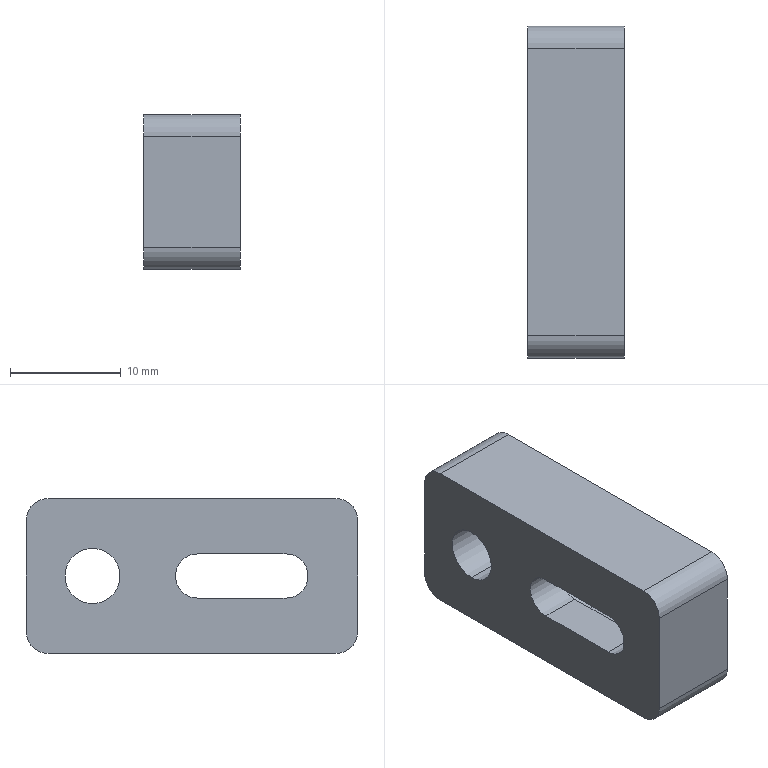Part | SolidWorks | features ICE 2, Extrusion 1, Fillet 1, HoleWzd 1 | 1 solid | 21 faces | box 8.7 x 30 x 14 mm | volume 2717 mm3 | plane 11 | cylinder 10 | commonest cylinder face diameters 4 x6 5 x2 8 x2
STEP:
#1=CARTESIAN_POINT('',(-4.35,9.,9.5));
#2=VERTEX_POINT('',#1);
#3=CARTESIAN_POINT('',(-4.35,9.,4.5));
#4=VERTEX_POINT('',#3);
#5=CARTESIAN_POINT('',(-4.35,9.,7.));
#6=DIRECTION('',(1.,0.,0.));
#7=DIRECTION('',(0.,0.,-1.));
#8=AXIS2_PLACEMENT_3D('',#5,#6,#7);
#9=CIRCLE('',#8,2.5);
#10=EDGE_CURVE('',#2,#4,#9,.T.);
#11=ORIENTED_EDGE('',*,*,#10,.F.);
#12=CARTESIAN_POINT('',(4.35,9.,9.5));
#13=VERTEX_POINT('',#12);
#14=CARTESIAN_POINT('',(4.35,9.,9.5));
#15=DIRECTION('',(1.,0.,0.));
#16=VECTOR('',#15,1000.);
#17=LINE('',#14,#16);
#18=EDGE_CURVE('',#2,#13,#17,.T.);
#19=ORIENTED_EDGE('',*,*,#18,.T.);
#20=CARTESIAN_POINT('',(4.35,9.,4.5));
#21=VERTEX_POINT('',#20);
#22=CARTESIAN_POINT('',(4.35,9.,7.));
#23=DIRECTION('',(1.,0.,0.));
#24=DIRECTION('',(0.,0.,-1.));
#25=AXIS2_PLACEMENT_3D('',#22,#23,#24);
#26=CIRCLE('',#25,2.5);
#27=EDGE_CURVE('',#13,#21,#26,.T.);
#28=ORIENTED_EDGE('',*,*,#27,.T.);
#29=CARTESIAN_POINT('',(4.35,9.,4.5));
#30=DIRECTION('',(1.,0.,0.));
#31=VECTOR('',#30,1000.);
#32=LINE('',#29,#31);
#33=EDGE_CURVE('',#4,#21,#32,.T.);
#34=ORIENTED_EDGE('',*,*,#33,.F.);
#35=EDGE_LOOP('',(#11,#19,#28,#34));
#36=FACE_OUTER_BOUND('',#35,.T.);
#37=CARTESIAN_POINT('',(4.35,9.,7.));
#38=DIRECTION('',(1.,0.,0.));
#39=DIRECTION('',(0.,0.,-1.));
#40=AXIS2_PLACEMENT_3D('',#37,#38,#39);
#41=CYLINDRICAL_SURFACE('',#40,2.5);
#42=ADVANCED_FACE('',(#36),#41,.F.);
#43=CARTESIAN_POINT('',(-0.65,-8.5,5.));
#44=VERTEX_POINT('',#43);
#45=CARTESIAN_POINT('',(-0.65,-8.5,9.));
#46=VERTEX_POINT('',#45);
#47=CARTESIAN_POINT('',(-0.65,-8.5,7.));
#48=DIRECTION('',(-1.,0.,0.));
#49=DIRECTION('',(0.,0.,-1.));
#50=AXIS2_PLACEMENT_3D('',#47,#48,#49);
#51=CIRCLE('',#50,2.);
#52=EDGE_CURVE('',#44,#46,#51,.T.);
#53=ORIENTED_EDGE('',*,*,#52,.F.);
#54=CARTESIAN_POINT('',(-4.35,-8.5,5.));
#55=VERTEX_POINT('',#54);
#56=CARTESIAN_POINT('',(-4.35,-8.5,5.));
#57=DIRECTION('',(1.,0.,0.));
#58=VECTOR('',#57,1000.);
#59=LINE('',#56,#58);
#60=EDGE_CURVE('',#55,#44,#59,.T.);
#61=ORIENTED_EDGE('',*,*,#60,.F.);
#62=CARTESIAN_POINT('',(-4.35,-8.5,9.));
#63=VERTEX_POINT('',#62);
#64=CARTESIAN_POINT('',(-4.35,-8.5,7.));
#65=DIRECTION('',(1.,0.,0.));
#66=DIRECTION('',(0.,0.,-1.));
#67=AXIS2_PLACEMENT_3D('',#64,#65,#66);
#68=CIRCLE('',#67,2.);
#69=EDGE_CURVE('',#63,#55,#68,.T.);
#70=ORIENTED_EDGE('',*,*,#69,.F.);
#71=CARTESIAN_POINT('',(-4.35,-8.5,9.));
#72=DIRECTION('',(1.,0.,0.));
#73=VECTOR('',#72,1000.);
#74=LINE('',#71,#73);
#75=EDGE_CURVE('',#63,#46,#74,.T.);
#76=ORIENTED_EDGE('',*,*,#75,.T.);
#77=EDGE_LOOP('',(#53,#61,#70,#76));
#78=FACE_OUTER_BOUND('',#77,.T.);
#79=CARTESIAN_POINT('',(-4.35,-8.5,7.));
#80=DIRECTION('',(1.,0.,0.));
#81=DIRECTION('',(0.,0.,-1.));
#82=AXIS2_PLACEMENT_3D('',#79,#80,#81);
#83=CYLINDRICAL_SURFACE('',#82,2.);
#84=ADVANCED_FACE('',(#78),#83,.F.);
#85=CARTESIAN_POINT('',(-0.65,-0.5,9.));
#86=VERTEX_POINT('',#85);
#87=CARTESIAN_POINT('',(-0.65,-8.5,9.));
#88=DIRECTION('',(0.,1.,0.));
#89=VECTOR('',#88,1000.);
#90=LINE('',#87,#89);
#91=EDGE_CURVE('',#46,#86,#90,.T.);
#92=ORIENTED_EDGE('',*,*,#91,.F.);
#93=ORIENTED_EDGE('',*,*,#75,.F.);
#94=CARTESIAN_POINT('',(-4.35,-0.5,9.));
#95=VERTEX_POINT('',#94);
#96=CARTESIAN_POINT('',(-4.35,-8.5,9.));
#97=DIRECTION('',(0.,-1.,0.));
#98=VECTOR('',#97,1000.);
#99=LINE('',#96,#98);
#100=EDGE_CURVE('',#95,#63,#99,.T.);
#101=ORIENTED_EDGE('',*,*,#100,.F.);
#102=CARTESIAN_POINT('',(-4.35,-0.5,9.));
#103=DIRECTION('',(1.,0.,0.));
#104=VECTOR('',#103,1000.);
#105=LINE('',#102,#104);
#106=EDGE_CURVE('',#95,#86,#105,.T.);
#107=ORIENTED_EDGE('',*,*,#106,.T.);
#108=EDGE_LOOP('',(#92,#93,#101,#107));
#109=FACE_OUTER_BOUND('',#108,.T.);
#110=CARTESIAN_POINT('',(-4.35,-8.5,9.));
#111=DIRECTION('',(0.,0.,1.));
#112=DIRECTION('',(1.,0.,0.));
#113=AXIS2_PLACEMENT_3D('',#110,#111,#112);
#114=PLANE('',#113);
#115=ADVANCED_FACE('',(#109),#114,.F.);
#116=CARTESIAN_POINT('',(-0.65,-0.5,5.));
#117=VERTEX_POINT('',#116);
#118=CARTESIAN_POINT('',(-0.65,-0.5,7.));
#119=DIRECTION('',(-1.,0.,0.));
#120=DIRECTION('',(0.,0.,-1.));
#121=AXIS2_PLACEMENT_3D('',#118,#119,#120);
#122=CIRCLE('',#121,2.);
#123=EDGE_CURVE('',#86,#117,#122,.T.);
#124=ORIENTED_EDGE('',*,*,#123,.F.);
#125=ORIENTED_EDGE('',*,*,#106,.F.);
#126=CARTESIAN_POINT('',(-4.35,-0.5,5.));
#127=VERTEX_POINT('',#126);
#128=CARTESIAN_POINT('',(-4.35,-0.5,7.));
#129=DIRECTION('',(1.,0.,0.));
#130=DIRECTION('',(0.,0.,-1.));
#131=AXIS2_PLACEMENT_3D('',#128,#129,#130);
#132=CIRCLE('',#131,2.);
#133=EDGE_CURVE('',#127,#95,#132,.T.);
#134=ORIENTED_EDGE('',*,*,#133,.F.);
#135=CARTESIAN_POINT('',(-4.35,-0.5,5.));
#136=DIRECTION('',(1.,0.,0.));
#137=VECTOR('',#136,1000.);
#138=LINE('',#135,#137);
#139=EDGE_CURVE('',#127,#117,#138,.T.);
#140=ORIENTED_EDGE('',*,*,#139,.T.);
#141=EDGE_LOOP('',(#124,#125,#134,#140));
#142=FACE_OUTER_BOUND('',#141,.T.);
#143=CARTESIAN_POINT('',(-4.35,-0.5,7.));
#144=DIRECTION('',(1.,0.,0.));
#145=DIRECTION('',(0.,0.,-1.));
#146=AXIS2_PLACEMENT_3D('',#143,#144,#145);
#147=CYLINDRICAL_SURFACE('',#146,2.);
#148=ADVANCED_FACE('',(#142),#147,.F.);
#149=CARTESIAN_POINT('',(-0.65,-8.5,5.));
#150=DIRECTION('',(0.,-1.,0.));
#151=VECTOR('',#150,1000.);
#152=LINE('',#149,#151);
#153=EDGE_CURVE('',#117,#44,#152,.T.);
#154=ORIENTED_EDGE('',*,*,#153,.F.);
#155=ORIENTED_EDGE('',*,*,#139,.F.);
#156=CARTESIAN_POINT('',(-4.35,-8.5,5.));
#157=DIRECTION('',(0.,1.,0.));
#158=VECTOR('',#157,1000.);
#159=LINE('',#156,#158);
#160=EDGE_CURVE('',#55,#127,#159,.T.);
#161=ORIENTED_EDGE('',*,*,#160,.F.);
#162=ORIENTED_EDGE('',*,*,#60,.T.);
#163=EDGE_LOOP('',(#154,#155,#161,#162));
#164=FACE_OUTER_BOUND('',#163,.T.);
#165=CARTESIAN_POINT('',(-4.35,-8.5,5.));
#166=DIRECTION('',(0.,0.,-1.));
#167=DIRECTION('',(-1.,0.,0.));
#168=AXIS2_PLACEMENT_3D('',#165,#166,#167);
#169=PLANE('',#168);
#170=ADVANCED_FACE('',(#164),#169,.F.);
#171=CARTESIAN_POINT('',(4.35,-0.5,11.));
#172=VERTEX_POINT('',#171);
#173=CARTESIAN_POINT('',(4.35,-8.5,11.));
#174=VERTEX_POINT('',#173);
#175=CARTESIAN_POINT('',(4.35,-0.5,11.));
#176=DIRECTION('',(0.,-1.,0.));
#177=VECTOR('',#176,1000.);
#178=LINE('',#175,#177);
#179=EDGE_CURVE('',#172,#174,#178,.T.);
#180=ORIENTED_EDGE('',*,*,#179,.F.);
#181=CARTESIAN_POINT('',(4.35,-0.5,3.));
#182=VERTEX_POINT('',#181);
#183=CARTESIAN_POINT('',(4.35,-0.5,7.));
#184=DIRECTION('',(1.,0.,0.));
#185=DIRECTION('',(0.,0.,-1.));
#186=AXIS2_PLACEMENT_3D('',#183,#184,#185);
#187=CIRCLE('',#186,4.);
#188=EDGE_CURVE('',#182,#172,#187,.T.);
#189=ORIENTED_EDGE('',*,*,#188,.F.);
#190=CARTESIAN_POINT('',(4.35,-8.5,3.));
#191=VERTEX_POINT('',#190);
#192=CARTESIAN_POINT('',(4.35,-0.5,3.));
#193=DIRECTION('',(0.,1.,0.));
#194=VECTOR('',#193,1000.);
#195=LINE('',#192,#194);
#196=EDGE_CURVE('',#191,#182,#195,.T.);
#197=ORIENTED_EDGE('',*,*,#196,.F.);
#198=CARTESIAN_POINT('',(4.35,-8.5,7.));
#199=DIRECTION('',(1.,0.,0.));
#200=DIRECTION('',(0.,0.,-1.));
#201=AXIS2_PLACEMENT_3D('',#198,#199,#200);
#202=CIRCLE('',#201,4.);
#203=EDGE_CURVE('',#174,#191,#202,.T.);
#204=ORIENTED_EDGE('',*,*,#203,.F.);
#205=EDGE_LOOP('',(#180,#189,#197,#204));
#206=FACE_BOUND('',#205,.T.);
#207=CARTESIAN_POINT('',(4.35,9.,7.));
#208=DIRECTION('',(1.,0.,0.));
#209=DIRECTION('',(0.,0.,-1.));
#210=AXIS2_PLACEMENT_3D('',#207,#208,#209);
#211=CIRCLE('',#210,2.5);
#212=EDGE_CURVE('',#21,#13,#211,.T.);
#213=ORIENTED_EDGE('',*,*,#212,.F.);
#214=ORIENTED_EDGE('',*,*,#27,.F.);
#215=EDGE_LOOP('',(#213,#214));
#216=FACE_BOUND('',#215,.T.);
#217=CARTESIAN_POINT('',(4.35,-15.,12.));
#218=VERTEX_POINT('',#217);
#219=CARTESIAN_POINT('',(4.35,-15.,2.));
#220=VERTEX_POINT('',#219);
#221=CARTESIAN_POINT('',(4.35,-15.,14.));
#222=DIRECTION('',(0.,0.,-1.));
#223=VECTOR('',#222,1000.);
#224=LINE('',#221,#223);
#225=EDGE_CURVE('',#218,#220,#224,.T.);
#226=ORIENTED_EDGE('',*,*,#225,.T.);
#227=CARTESIAN_POINT('',(4.35,-13.,0.));
#228=VERTEX_POINT('',#227);
#229=CARTESIAN_POINT('',(4.35,-13.,2.));
#230=DIRECTION('',(1.,0.,0.));
#231=DIRECTION('',(0.,-1.,0.));
#232=AXIS2_PLACEMENT_3D('',#229,#230,#231);
#233=CIRCLE('',#232,2.);
#234=EDGE_CURVE('',#220,#228,#233,.T.);
#235=ORIENTED_EDGE('',*,*,#234,.T.);
#236=CARTESIAN_POINT('',(4.35,13.,0.));
#237=VERTEX_POINT('',#236);
#238=CARTESIAN_POINT('',(4.35,15.,0.));
#239=DIRECTION('',(0.,1.,0.));
#240=VECTOR('',#239,1000.);
#241=LINE('',#238,#240);
#242=EDGE_CURVE('',#228,#237,#241,.T.);
#243=ORIENTED_EDGE('',*,*,#242,.T.);
#244=CARTESIAN_POINT('',(4.35,15.,2.));
#245=VERTEX_POINT('',#244);
#246=CARTESIAN_POINT('',(4.35,13.,2.));
#247=DIRECTION('',(1.,0.,0.));
#248=DIRECTION('',(0.,-1.,0.));
#249=AXIS2_PLACEMENT_3D('',#246,#247,#248);
#250=CIRCLE('',#249,2.);
#251=EDGE_CURVE('',#237,#245,#250,.T.);
#252=ORIENTED_EDGE('',*,*,#251,.T.);
#253=CARTESIAN_POINT('',(4.35,15.,12.));
#254=VERTEX_POINT('',#253);
#255=CARTESIAN_POINT('',(4.35,15.,14.));
#256=DIRECTION('',(0.,0.,-1.));
#257=VECTOR('',#256,1000.);
#258=LINE('',#255,#257);
#259=EDGE_CURVE('',#254,#245,#258,.T.);
#260=ORIENTED_EDGE('',*,*,#259,.F.);
#261=CARTESIAN_POINT('',(4.35,13.,14.));
#262=VERTEX_POINT('',#261);
#263=CARTESIAN_POINT('',(4.35,13.,12.));
#264=DIRECTION('',(1.,0.,0.));
#265=DIRECTION('',(0.,-1.,0.));
#266=AXIS2_PLACEMENT_3D('',#263,#264,#265);
#267=CIRCLE('',#266,2.);
#268=EDGE_CURVE('',#254,#262,#267,.T.);
#269=ORIENTED_EDGE('',*,*,#268,.T.);
#270=CARTESIAN_POINT('',(4.35,-13.,14.));
#271=VERTEX_POINT('',#270);
#272=CARTESIAN_POINT('',(4.35,15.,14.));
#273=DIRECTION('',(0.,1.,0.));
#274=VECTOR('',#273,1000.);
#275=LINE('',#272,#274);
#276=EDGE_CURVE('',#271,#262,#275,.T.);
#277=ORIENTED_EDGE('',*,*,#276,.F.);
#278=CARTESIAN_POINT('',(4.35,-13.,12.));
#279=DIRECTION('',(1.,0.,0.));
#280=DIRECTION('',(0.,-1.,0.));
#281=AXIS2_PLACEMENT_3D('',#278,#279,#280);
#282=CIRCLE('',#281,2.);
#283=EDGE_CURVE('',#271,#218,#282,.T.);
#284=ORIENTED_EDGE('',*,*,#283,.T.);
#285=EDGE_LOOP('',(#226,#235,#243,#252,#260,#269,#277,#284));
#286=FACE_OUTER_BOUND('',#285,.T.);
#287=CARTESIAN_POINT('',(4.35,15.,14.));
#288=DIRECTION('',(-1.,0.,0.));
#289=DIRECTION('',(0.,-1.,0.));
#290=AXIS2_PLACEMENT_3D('',#287,#288,#289);
#291=PLANE('',#290);
#292=ADVANCED_FACE('',(#206,#216,#286),#291,.F.);
#293=CARTESIAN_POINT('',(-4.35,15.,12.));
#294=VERTEX_POINT('',#293);
#295=CARTESIAN_POINT('',(-4.35,15.,2.));
#296=VERTEX_POINT('',#295);
#297=CARTESIAN_POINT('',(-4.35,15.,14.));
#298=DIRECTION('',(0.,0.,-1.));
#299=VECTOR('',#298,1000.);
#300=LINE('',#297,#299);
#301=EDGE_CURVE('',#294,#296,#300,.T.);
#302=ORIENTED_EDGE('',*,*,#301,.F.);
#303=CARTESIAN_POINT('',(4.35,15.,12.));
#304=DIRECTION('',(1.,0.,0.));
#305=VECTOR('',#304,1000.);
#306=LINE('',#303,#305);
#307=EDGE_CURVE('',#294,#254,#306,.T.);
#308=ORIENTED_EDGE('',*,*,#307,.T.);
#309=ORIENTED_EDGE('',*,*,#259,.T.);
#310=CARTESIAN_POINT('',(-4.35,15.,2.));
#311=DIRECTION('',(-1.,0.,0.));
#312=VECTOR('',#311,1000.);
#313=LINE('',#310,#312);
#314=EDGE_CURVE('',#245,#296,#313,.T.);
#315=ORIENTED_EDGE('',*,*,#314,.T.);
#316=EDGE_LOOP('',(#302,#308,#309,#315));
#317=FACE_OUTER_BOUND('',#316,.T.);
#318=CARTESIAN_POINT('',(-4.35,15.,14.));
#319=DIRECTION('',(0.,-1.,0.));
#320=DIRECTION('',(0.,0.,-1.));
#321=AXIS2_PLACEMENT_3D('',#318,#319,#320);
#322=PLANE('',#321);
#323=ADVANCED_FACE('',(#317),#322,.F.);
#324=ORIENTED_EDGE('',*,*,#100,.T.);
#325=ORIENTED_EDGE('',*,*,#69,.T.);
#326=ORIENTED_EDGE('',*,*,#160,.T.);
#327=ORIENTED_EDGE('',*,*,#133,.T.);
#328=EDGE_LOOP('',(#324,#325,#326,#327));
#329=FACE_BOUND('',#328,.T.);
#330=CARTESIAN_POINT('',(-4.35,9.,7.));
#331=DIRECTION('',(1.,0.,0.));
#332=DIRECTION('',(0.,0.,-1.));
#333=AXIS2_PLACEMENT_3D('',#330,#331,#332);
#334=CIRCLE('',#333,2.5);
#335=EDGE_CURVE('',#4,#2,#334,.T.);
#336=ORIENTED_EDGE('',*,*,#335,.T.);
#337=ORIENTED_EDGE('',*,*,#10,.T.);
#338=EDGE_LOOP('',(#336,#337));
#339=FACE_BOUND('',#338,.T.);
#340=CARTESIAN_POINT('',(-4.35,13.,0.));
#341=VERTEX_POINT('',#340);
#342=CARTESIAN_POINT('',(-4.35,-13.,0.));
#343=VERTEX_POINT('',#342);
#344=CARTESIAN_POINT('',(-4.35,15.,0.));
#345=DIRECTION('',(0.,-1.,0.));
#346=VECTOR('',#345,1000.);
#347=LINE('',#344,#346);
#348=EDGE_CURVE('',#341,#343,#347,.T.);
#349=ORIENTED_EDGE('',*,*,#348,.T.);
#350=CARTESIAN_POINT('',(-4.35,-15.,2.));
#351=VERTEX_POINT('',#350);
#352=CARTESIAN_POINT('',(-4.35,-13.,2.));
#353=DIRECTION('',(-1.,0.,0.));
#354=DIRECTION('',(0.,1.,0.));
#355=AXIS2_PLACEMENT_3D('',#352,#353,#354);
#356=CIRCLE('',#355,2.);
#357=EDGE_CURVE('',#343,#351,#356,.T.);
#358=ORIENTED_EDGE('',*,*,#357,.T.);
#359=CARTESIAN_POINT('',(-4.35,-15.,12.));
#360=VERTEX_POINT('',#359);
#361=CARTESIAN_POINT('',(-4.35,-15.,14.));
#362=DIRECTION('',(0.,0.,-1.));
#363=VECTOR('',#362,1000.);
#364=LINE('',#361,#363);
#365=EDGE_CURVE('',#360,#351,#364,.T.);
#366=ORIENTED_EDGE('',*,*,#365,.F.);
#367=CARTESIAN_POINT('',(-4.35,-13.,14.));
#368=VERTEX_POINT('',#367);
#369=CARTESIAN_POINT('',(-4.35,-13.,12.));
#370=DIRECTION('',(-1.,0.,0.));
#371=DIRECTION('',(0.,1.,0.));
#372=AXIS2_PLACEMENT_3D('',#369,#370,#371);
#373=CIRCLE('',#372,2.);
#374=EDGE_CURVE('',#360,#368,#373,.T.);
#375=ORIENTED_EDGE('',*,*,#374,.T.);
#376=CARTESIAN_POINT('',(-4.35,13.,14.));
#377=VERTEX_POINT('',#376);
#378=CARTESIAN_POINT('',(-4.35,15.,14.));
#379=DIRECTION('',(0.,-1.,0.));
#380=VECTOR('',#379,1000.);
#381=LINE('',#378,#380);
#382=EDGE_CURVE('',#377,#368,#381,.T.);
#383=ORIENTED_EDGE('',*,*,#382,.F.);
#384=CARTESIAN_POINT('',(-4.35,13.,12.));
#385=DIRECTION('',(-1.,0.,0.));
#386=DIRECTION('',(0.,1.,0.));
#387=AXIS2_PLACEMENT_3D('',#384,#385,#386);
#388=CIRCLE('',#387,2.);
#389=EDGE_CURVE('',#377,#294,#388,.T.);
#390=ORIENTED_EDGE('',*,*,#389,.T.);
#391=ORIENTED_EDGE('',*,*,#301,.T.);
#392=CARTESIAN_POINT('',(-4.35,13.,2.));
#393=DIRECTION('',(-1.,0.,0.));
#394=DIRECTION('',(0.,1.,0.));
#395=AXIS2_PLACEMENT_3D('',#392,#393,#394);
#396=CIRCLE('',#395,2.);
#397=EDGE_CURVE('',#296,#341,#396,.T.);
#398=ORIENTED_EDGE('',*,*,#397,.T.);
#399=EDGE_LOOP('',(#349,#358,#366,#375,#383,#390,#391,#398));
#400=FACE_OUTER_BOUND('',#399,.T.);
#401=CARTESIAN_POINT('',(-4.35,15.,14.));
#402=DIRECTION('',(1.,0.,0.));
#403=DIRECTION('',(0.,1.,0.));
#404=AXIS2_PLACEMENT_3D('',#401,#402,#403);
#405=PLANE('',#404);
#406=ADVANCED_FACE('',(#329,#339,#400),#405,.F.);
#407=ORIENTED_EDGE('',*,*,#365,.T.);
#408=CARTESIAN_POINT('',(-4.35,-15.,2.));
#409=DIRECTION('',(1.,0.,0.));
#410=VECTOR('',#409,1000.);
#411=LINE('',#408,#410);
#412=EDGE_CURVE('',#351,#220,#411,.T.);
#413=ORIENTED_EDGE('',*,*,#412,.T.);
#414=ORIENTED_EDGE('',*,*,#225,.F.);
#415=CARTESIAN_POINT('',(-4.35,-15.,12.));
#416=DIRECTION('',(-1.,0.,0.));
#417=VECTOR('',#416,1000.);
#418=LINE('',#415,#417);
#419=EDGE_CURVE('',#218,#360,#418,.T.);
#420=ORIENTED_EDGE('',*,*,#419,.T.);
#421=EDGE_LOOP('',(#407,#413,#414,#420));
#422=FACE_OUTER_BOUND('',#421,.T.);
#423=CARTESIAN_POINT('',(-4.35,-15.,14.));
#424=DIRECTION('',(0.,1.,0.));
#425=DIRECTION('',(0.,0.,1.));
#426=AXIS2_PLACEMENT_3D('',#423,#424,#425);
#427=PLANE('',#426);
#428=ADVANCED_FACE('',(#422),#427,.F.);
#429=ORIENTED_EDGE('',*,*,#382,.T.);
#430=CARTESIAN_POINT('',(4.35,-13.,14.));
#431=DIRECTION('',(1.,0.,0.));
#432=VECTOR('',#431,1000.);
#433=LINE('',#430,#432);
#434=EDGE_CURVE('',#368,#271,#433,.T.);
#435=ORIENTED_EDGE('',*,*,#434,.T.);
#436=ORIENTED_EDGE('',*,*,#276,.T.);
#437=CARTESIAN_POINT('',(-4.35,13.,14.));
#438=DIRECTION('',(-1.,0.,0.));
#439=VECTOR('',#438,1000.);
#440=LINE('',#437,#439);
#441=EDGE_CURVE('',#262,#377,#440,.T.);
#442=ORIENTED_EDGE('',*,*,#441,.T.);
#443=EDGE_LOOP('',(#429,#435,#436,#442));
#444=FACE_OUTER_BOUND('',#443,.T.);
#445=CARTESIAN_POINT('',(0.,0.,14.));
#446=DIRECTION('',(0.,0.,1.));
#447=DIRECTION('',(1.,0.,0.));
#448=AXIS2_PLACEMENT_3D('',#445,#446,#447);
#449=PLANE('',#448);
#450=ADVANCED_FACE('',(#444),#449,.T.);
#451=ORIENTED_EDGE('',*,*,#242,.F.);
#452=CARTESIAN_POINT('',(0.,-13.,0.));
#453=DIRECTION('',(-1.,0.,0.));
#454=VECTOR('',#453,1000.);
#455=LINE('',#452,#454);
#456=EDGE_CURVE('',#228,#343,#455,.T.);
#457=ORIENTED_EDGE('',*,*,#456,.T.);
#458=ORIENTED_EDGE('',*,*,#348,.F.);
#459=CARTESIAN_POINT('',(0.,13.,0.));
#460=DIRECTION('',(1.,0.,0.));
#461=VECTOR('',#460,1000.);
#462=LINE('',#459,#461);
#463=EDGE_CURVE('',#341,#237,#462,.T.);
#464=ORIENTED_EDGE('',*,*,#463,.T.);
#465=EDGE_LOOP('',(#451,#457,#458,#464));
#466=FACE_OUTER_BOUND('',#465,.T.);
#467=CARTESIAN_POINT('',(0.,0.,0.));
#468=DIRECTION('',(0.,0.,1.));
#469=DIRECTION('',(1.,0.,0.));
#470=AXIS2_PLACEMENT_3D('',#467,#468,#469);
#471=PLANE('',#470);
#472=ADVANCED_FACE('',(#466),#471,.F.);
#473=ORIENTED_EDGE('',*,*,#18,.F.);
#474=ORIENTED_EDGE('',*,*,#335,.F.);
#475=ORIENTED_EDGE('',*,*,#33,.T.);
#476=ORIENTED_EDGE('',*,*,#212,.T.);
#477=EDGE_LOOP('',(#473,#474,#475,#476));
#478=FACE_OUTER_BOUND('',#477,.T.);
#479=CARTESIAN_POINT('',(4.35,9.,7.));
#480=DIRECTION('',(1.,0.,0.));
#481=DIRECTION('',(0.,0.,-1.));
#482=AXIS2_PLACEMENT_3D('',#479,#480,#481);
#483=CYLINDRICAL_SURFACE('',#482,2.5);
#484=ADVANCED_FACE('',(#478),#483,.F.);
#485=CARTESIAN_POINT('',(-0.65,-0.5,3.));
#486=VERTEX_POINT('',#485);
#487=CARTESIAN_POINT('',(-0.65,-0.5,11.));
#488=VERTEX_POINT('',#487);
#489=CARTESIAN_POINT('',(-0.65,-0.5,7.));
#490=DIRECTION('',(1.,0.,0.));
#491=DIRECTION('',(0.,0.,-1.));
#492=AXIS2_PLACEMENT_3D('',#489,#490,#491);
#493=CIRCLE('',#492,4.);
#494=EDGE_CURVE('',#486,#488,#493,.T.);
#495=ORIENTED_EDGE('',*,*,#494,.T.);
#496=CARTESIAN_POINT('',(-0.65,-8.5,11.));
#497=VERTEX_POINT('',#496);
#498=CARTESIAN_POINT('',(-0.65,-0.5,11.));
#499=DIRECTION('',(0.,-1.,0.));
#500=VECTOR('',#499,1000.);
#501=LINE('',#498,#500);
#502=EDGE_CURVE('',#488,#497,#501,.T.);
#503=ORIENTED_EDGE('',*,*,#502,.T.);
#504=CARTESIAN_POINT('',(-0.65,-8.5,3.));
#505=VERTEX_POINT('',#504);
#506=CARTESIAN_POINT('',(-0.65,-8.5,7.));
#507=DIRECTION('',(1.,0.,0.));
#508=DIRECTION('',(0.,0.,-1.));
#509=AXIS2_PLACEMENT_3D('',#506,#507,#508);
#510=CIRCLE('',#509,4.);
#511=EDGE_CURVE('',#497,#505,#510,.T.);
#512=ORIENTED_EDGE('',*,*,#511,.T.);
#513=CARTESIAN_POINT('',(-0.65,-0.5,3.));
#514=DIRECTION('',(0.,1.,0.));
#515=VECTOR('',#514,1000.);
#516=LINE('',#513,#515);
#517=EDGE_CURVE('',#505,#486,#516,.T.);
#518=ORIENTED_EDGE('',*,*,#517,.T.);
#519=EDGE_LOOP('',(#495,#503,#512,#518));
#520=FACE_OUTER_BOUND('',#519,.T.);
#521=ORIENTED_EDGE('',*,*,#52,.T.);
#522=ORIENTED_EDGE('',*,*,#91,.T.);
#523=ORIENTED_EDGE('',*,*,#123,.T.);
#524=ORIENTED_EDGE('',*,*,#153,.T.);
#525=EDGE_LOOP('',(#521,#522,#523,#524));
#526=FACE_BOUND('',#525,.T.);
#527=CARTESIAN_POINT('',(-0.65,-0.5,7.));
#528=DIRECTION('',(1.,0.,0.));
#529=DIRECTION('',(0.,0.,-1.));
#530=AXIS2_PLACEMENT_3D('',#527,#528,#529);
#531=PLANE('',#530);
#532=ADVANCED_FACE('',(#520,#526),#531,.T.);
#533=ORIENTED_EDGE('',*,*,#188,.T.);
#534=CARTESIAN_POINT('',(-0.65,-0.5,11.));
#535=DIRECTION('',(1.,0.,0.));
#536=VECTOR('',#535,1000.);
#537=LINE('',#534,#536);
#538=EDGE_CURVE('',#488,#172,#537,.T.);
#539=ORIENTED_EDGE('',*,*,#538,.F.);
#540=ORIENTED_EDGE('',*,*,#494,.F.);
#541=CARTESIAN_POINT('',(-0.65,-0.5,3.));
#542=DIRECTION('',(1.,0.,0.));
#543=VECTOR('',#542,1000.);
#544=LINE('',#541,#543);
#545=EDGE_CURVE('',#486,#182,#544,.T.);
#546=ORIENTED_EDGE('',*,*,#545,.T.);
#547=EDGE_LOOP('',(#533,#539,#540,#546));
#548=FACE_OUTER_BOUND('',#547,.T.);
#549=CARTESIAN_POINT('',(-0.65,-0.5,7.));
#550=DIRECTION('',(1.,0.,0.));
#551=DIRECTION('',(0.,0.,-1.));
#552=AXIS2_PLACEMENT_3D('',#549,#550,#551);
#553=CYLINDRICAL_SURFACE('',#552,4.);
#554=ADVANCED_FACE('',(#548),#553,.F.);
#555=ORIENTED_EDGE('',*,*,#196,.T.);
#556=ORIENTED_EDGE('',*,*,#545,.F.);
#557=ORIENTED_EDGE('',*,*,#517,.F.);
#558=CARTESIAN_POINT('',(-0.65,-8.5,3.));
#559=DIRECTION('',(1.,0.,0.));
#560=VECTOR('',#559,1000.);
#561=LINE('',#558,#560);
#562=EDGE_CURVE('',#505,#191,#561,.T.);
#563=ORIENTED_EDGE('',*,*,#562,.T.);
#564=EDGE_LOOP('',(#555,#556,#557,#563));
#565=FACE_OUTER_BOUND('',#564,.T.);
#566=CARTESIAN_POINT('',(-0.65,-0.5,3.));
#567=DIRECTION('',(0.,0.,-1.));
#568=DIRECTION('',(0.,1.,0.));
#569=AXIS2_PLACEMENT_3D('',#566,#567,#568);
#570=PLANE('',#569);
#571=ADVANCED_FACE('',(#565),#570,.F.);
#572=ORIENTED_EDGE('',*,*,#203,.T.);
#573=ORIENTED_EDGE('',*,*,#562,.F.);
#574=ORIENTED_EDGE('',*,*,#511,.F.);
#575=CARTESIAN_POINT('',(-0.65,-8.5,11.));
#576=DIRECTION('',(1.,0.,0.));
#577=VECTOR('',#576,1000.);
#578=LINE('',#575,#577);
#579=EDGE_CURVE('',#497,#174,#578,.T.);
#580=ORIENTED_EDGE('',*,*,#579,.T.);
#581=EDGE_LOOP('',(#572,#573,#574,#580));
#582=FACE_OUTER_BOUND('',#581,.T.);
#583=CARTESIAN_POINT('',(-0.65,-8.5,7.));
#584=DIRECTION('',(1.,0.,0.));
#585=DIRECTION('',(0.,0.,-1.));
#586=AXIS2_PLACEMENT_3D('',#583,#584,#585);
#587=CYLINDRICAL_SURFACE('',#586,4.);
#588=ADVANCED_FACE('',(#582),#587,.F.);
#589=ORIENTED_EDGE('',*,*,#179,.T.);
#590=ORIENTED_EDGE('',*,*,#579,.F.);
#591=ORIENTED_EDGE('',*,*,#502,.F.);
#592=ORIENTED_EDGE('',*,*,#538,.T.);
#593=EDGE_LOOP('',(#589,#590,#591,#592));
#594=FACE_OUTER_BOUND('',#593,.T.);
#595=CARTESIAN_POINT('',(-0.65,-0.5,11.));
#596=DIRECTION('',(0.,0.,1.));
#597=DIRECTION('',(1.,0.,0.));
#598=AXIS2_PLACEMENT_3D('',#595,#596,#597);
#599=PLANE('',#598);
#600=ADVANCED_FACE('',(#594),#599,.F.);
#601=ORIENTED_EDGE('',*,*,#357,.F.);
#602=ORIENTED_EDGE('',*,*,#456,.F.);
#603=ORIENTED_EDGE('',*,*,#234,.F.);
#604=ORIENTED_EDGE('',*,*,#412,.F.);
#605=EDGE_LOOP('',(#601,#602,#603,#604));
#606=FACE_OUTER_BOUND('',#605,.T.);
#607=CARTESIAN_POINT('',(-4.35,-13.,2.));
#608=DIRECTION('',(1.,0.,0.));
#609=DIRECTION('',(0.,0.,-1.));
#610=AXIS2_PLACEMENT_3D('',#607,#608,#609);
#611=CYLINDRICAL_SURFACE('',#610,2.);
#612=ADVANCED_FACE('',(#606),#611,.T.);
#613=ORIENTED_EDGE('',*,*,#374,.F.);
#614=ORIENTED_EDGE('',*,*,#419,.F.);
#615=ORIENTED_EDGE('',*,*,#283,.F.);
#616=ORIENTED_EDGE('',*,*,#434,.F.);
#617=EDGE_LOOP('',(#613,#614,#615,#616));
#618=FACE_OUTER_BOUND('',#617,.T.);
#619=CARTESIAN_POINT('',(0.,-13.,12.));
#620=DIRECTION('',(-1.,0.,0.));
#621=DIRECTION('',(0.,0.,1.));
#622=AXIS2_PLACEMENT_3D('',#619,#620,#621);
#623=CYLINDRICAL_SURFACE('',#622,2.);
#624=ADVANCED_FACE('',(#618),#623,.T.);
#625=ORIENTED_EDGE('',*,*,#268,.F.);
#626=ORIENTED_EDGE('',*,*,#307,.F.);
#627=ORIENTED_EDGE('',*,*,#389,.F.);
#628=ORIENTED_EDGE('',*,*,#441,.F.);
#629=EDGE_LOOP('',(#625,#626,#627,#628));
#630=FACE_OUTER_BOUND('',#629,.T.);
#631=CARTESIAN_POINT('',(0.,13.,12.));
#632=DIRECTION('',(1.,0.,0.));
#633=DIRECTION('',(0.,0.,-1.));
#634=AXIS2_PLACEMENT_3D('',#631,#632,#633);
#635=CYLINDRICAL_SURFACE('',#634,2.);
#636=ADVANCED_FACE('',(#630),#635,.T.);
#637=ORIENTED_EDGE('',*,*,#251,.F.);
#638=ORIENTED_EDGE('',*,*,#463,.F.);
#639=ORIENTED_EDGE('',*,*,#397,.F.);
#640=ORIENTED_EDGE('',*,*,#314,.F.);
#641=EDGE_LOOP('',(#637,#638,#639,#640));
#642=FACE_OUTER_BOUND('',#641,.T.);
#643=CARTESIAN_POINT('',(-4.35,13.,2.));
#644=DIRECTION('',(-1.,0.,0.));
#645=DIRECTION('',(0.,0.,1.));
#646=AXIS2_PLACEMENT_3D('',#643,#644,#645);
#647=CYLINDRICAL_SURFACE('',#646,2.);
#648=ADVANCED_FACE('',(#642),#647,.T.);
#649=CLOSED_SHELL('',(#42,#84,#115,#148,#170,#292,#323,#406,#428,#450,#472,#484,#532,#554,#571,#588,#600,#612,#624,#636,#648));
#650=MANIFOLD_SOLID_BREP('',#649);
#651=CARTESIAN_POINT('',(0.,0.,0.));
#652=DIRECTION('',(0.,0.,1.));
#653=DIRECTION('',(1.,0.,0.));
#654=AXIS2_PLACEMENT_3D('',#651,#652,#653);
#655=(LENGTH_UNIT()NAMED_UNIT(*)SI_UNIT(.MILLI.,.METRE.));
#656=UNCERTAINTY_MEASURE_WITH_UNIT(LENGTH_MEASURE(0.00001),#655,'','');
#657=(NAMED_UNIT(*)PLANE_ANGLE_UNIT()SI_UNIT($,.RADIAN.));
#658=(NAMED_UNIT(*)SI_UNIT($,.STERADIAN.)SOLID_ANGLE_UNIT());
#659=(GEOMETRIC_REPRESENTATION_CONTEXT(3)GLOBAL_UNCERTAINTY_ASSIGNED_CONTEXT((#656))GLOBAL_UNIT_ASSIGNED_CONTEXT((#655,#657,#658))REPRESENTATION_CONTEXT('',''));
#660=ADVANCED_BREP_SHAPE_REPRESENTATION('',(#650,#654),#659);